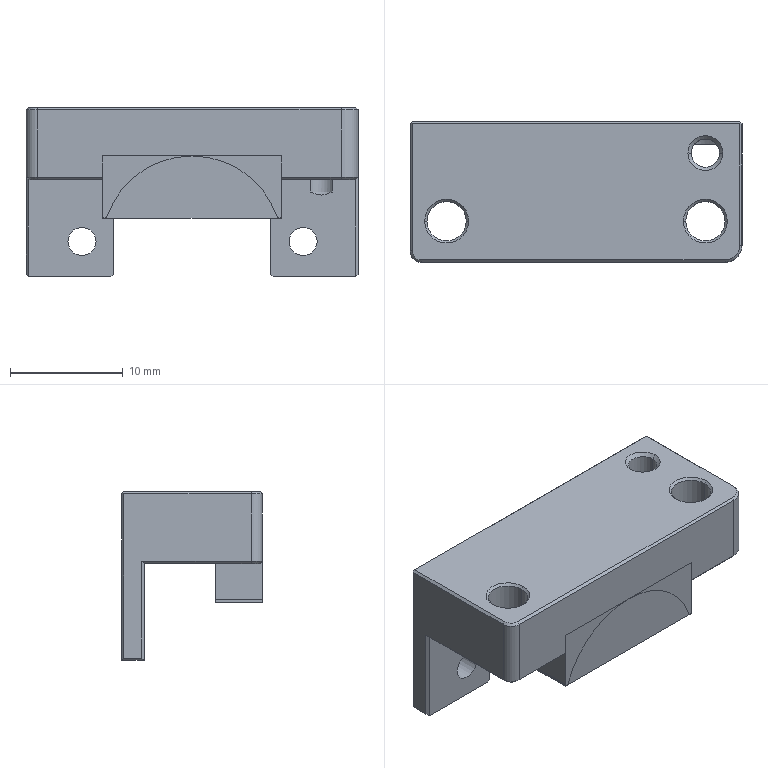NC program | NX | posted with a generic post | part box 29.5 x 12.5 x 15 mm
Whole program:
N10 G17 G21 G94 G90
(ZLEVEL_PROFILE_1_COPY_COPY_COPY , TOOL : D4)
N12 T17 M6
N14 G54
N16 G17 G0 G90 X10.45 Y-9.159 B0. C0. S9500 M3
N18 G43 Z30. H17
N20 Z-0.382
N22 G94 G1 X10.25 Y-9.275 F2000.
N24 G3 X10.05 Y-9.621 R0.4
N26 G2 X5.576 Y-10.372 R2.3
N28 G3 X-5.576 Y-10.372 R5.9
N30 G2 X-10.05 Y-9.621 R2.3
N32 G3 X-10.25 Y-9.275 R0.4
N34 G1 X-10.45 Y-9.159
N36 G0 Z-0.764
N38 G1 X-10.25 Y-9.275
N40 G2 X-10.05 Y-9.621 R0.4
N42 G3 X-5.576 Y-10.372 R2.3
N44 G2 X5.576 Y-10.372 R5.9
N46 G3 X10.05 Y-9.621 R2.3
N48 G2 X10.25 Y-9.275 R0.4
N50 G1 X10.45 Y-9.159
N52 G0 Z-1.145
N54 G1 X10.25 Y-9.275
N56 G3 X10.05 Y-9.621 R0.4
N58 G2 X5.576 Y-10.372 R2.3
N60 G3 X-5.576 Y-10.372 R5.9
N62 G2 X-10.05 Y-9.621 R2.3
N64 G3 X-10.25 Y-9.275 R0.4
N66 G1 X-10.45 Y-9.159
N68 G0 Z-1.527
N70 G1 X-10.25 Y-9.275
N72 G2 X-10.05 Y-9.621 R0.4
N74 G3 X-5.576 Y-10.372 R2.3
N76 G2 X5.576 Y-10.372 R5.9
N78 G3 X10.05 Y-9.621 R2.3
N80 G2 X10.25 Y-9.275 R0.4
N82 G1 X10.45 Y-9.159
N84 G0 Z-1.909
N86 G1 X10.25 Y-9.275
N88 G3 X10.05 Y-9.621 R0.4
N90 G2 X5.576 Y-10.372 R2.3
N92 G3 X-5.576 Y-10.372 R5.9
N94 G2 X-10.05 Y-9.621 R2.3
N96 G3 X-10.25 Y-9.275 R0.4
N98 G1 X-10.45 Y-9.159
N100 G0 Z-2.291
N102 G1 X-10.25 Y-9.275
N104 G2 X-10.05 Y-9.621 R0.4
N106 G3 X-5.576 Y-10.372 R2.3
N108 G2 X5.576 Y-10.372 R5.9
N110 G3 X10.05 Y-9.621 R2.3
N112 G2 X10.25 Y-9.275 R0.4
N114 G1 X10.45 Y-9.159
N116 G0 Z-2.673
N118 G1 X10.25 Y-9.275
N120 G3 X10.05 Y-9.621 R0.4
N122 G2 X5.576 Y-10.372 R2.3
N124 G3 X-5.576 Y-10.372 R5.9
N126 G2 X-10.05 Y-9.621 R2.3
N128 G3 X-10.25 Y-9.275 R0.4
N130 G1 X-10.45 Y-9.159
N132 G0 Z-3.055
N134 G1 X-10.25 Y-9.275
N136 G2 X-10.05 Y-9.621 R0.4
N138 G3 X-5.576 Y-10.372 R2.3
N140 G2 X5.576 Y-10.372 R5.9
N142 G3 X10.05 Y-9.621 R2.3
N144 G2 X10.25 Y-9.275 R0.4
N146 G1 X10.45 Y-9.159
N148 G0 Z-3.436
N150 G1 X10.25 Y-9.275
N152 G3 X10.05 Y-9.621 R0.4
N154 G2 X5.576 Y-10.372 R2.3
N156 G3 X-5.576 Y-10.372 R5.9
N158 G2 X-10.05 Y-9.621 R2.3
N160 G3 X-10.25 Y-9.275 R0.4
N162 G1 X-10.45 Y-9.159
N164 G0 Z-3.818
N166 G1 X-10.25 Y-9.275
N168 G2 X-10.05 Y-9.621 R0.4
N170 G3 X-5.576 Y-10.372 R2.3
N172 G2 X5.576 Y-10.372 R5.9
N174 G3 X10.05 Y-9.621 R2.3
N176 G2 X10.25 Y-9.275 R0.4
N178 G1 X10.45 Y-9.159
N180 G0 Z-4.2
N182 G1 X10.25 Y-9.275
N184 G3 X10.05 Y-9.621 R0.4
N186 G2 X5.576 Y-10.372 R2.3
N188 G3 X-5.576 Y-10.372 R5.9
N190 G2 X-10.05 Y-9.621 R2.3
N192 G3 X-10.25 Y-9.275 R0.4
N194 G1 X-10.45 Y-9.159
N196 G0 Z30.
(ZLEVEL_PROFILE_1_COPY_COPY_1 , TOOL : D4)
N198 X10.35
N200 Z-3.2
N202 G1 Z-4.2 F1000.
N204 X10.15 Y-9.275
N206 G3 X9.95 Y-9.621 R0.4
N208 G2 X5.671 Y-10.34 R2.2
N210 G3 X-5.671 Y-10.34 R6.
N212 G2 X-9.95 Y-9.621 R2.2
N214 G3 X-10.15 Y-9.275 R0.4
N216 G1 X-10.35 Y-9.159
N218 Z-3.2
N220 G0 Z30.
N222 M5
(PLANAR_MILL , TOOL : D6A45)
N224 T01 M6
N226 G54
N228 G17 G0 G90 X-1.27 Y2.1 B0. C0. S9500 M3
N230 G43 Z30. H1
N232 Z0.5
N234 G94 G1 Z-1. F1250.
N236 X-0.866 Y1.4
N238 G3 X0. Y0.9 R1.
N240 G1 X14.509
N242 G2 X15.216 Y0.607 R1.
N244 G1 X15.357 Y0.466
N246 G2 X15.65 Y-0.241 R1.
N248 G1 Y-6.159
N250 G2 X15.357 Y-6.866 R1.
N252 G1 X15.216 Y-7.007
N254 G2 X14.509 Y-7.3 R1.
N256 G1 X13.25
N258 X8.85
N260 Y-9.621
N262 G2 X6.71 Y-9.98 R1.1
N264 G3 X-6.71 Y-9.98 R7.1
N266 G2 X-8.85 Y-9.621 R1.1
N268 G1 Y-7.3
N270 X-14.509
N272 G2 X-15.216 Y-7.007 R1.
N274 G1 X-15.357 Y-6.866
N276 G2 X-15.65 Y-6.159 R1.
N278 G1 Y-0.241
N280 G2 X-15.357 Y0.466 R1.
N282 G1 X-15.216 Y0.607
N284 G2 X-14.509 Y0.9 R1.
N286 G1 X-13.75
N288 X0.
N290 G3 X0.866 Y1.4 R1.
N292 G1 X1.27 Y2.1
N294 Z0.5
N296 G0 Z30.
N298 M5
N300 M2